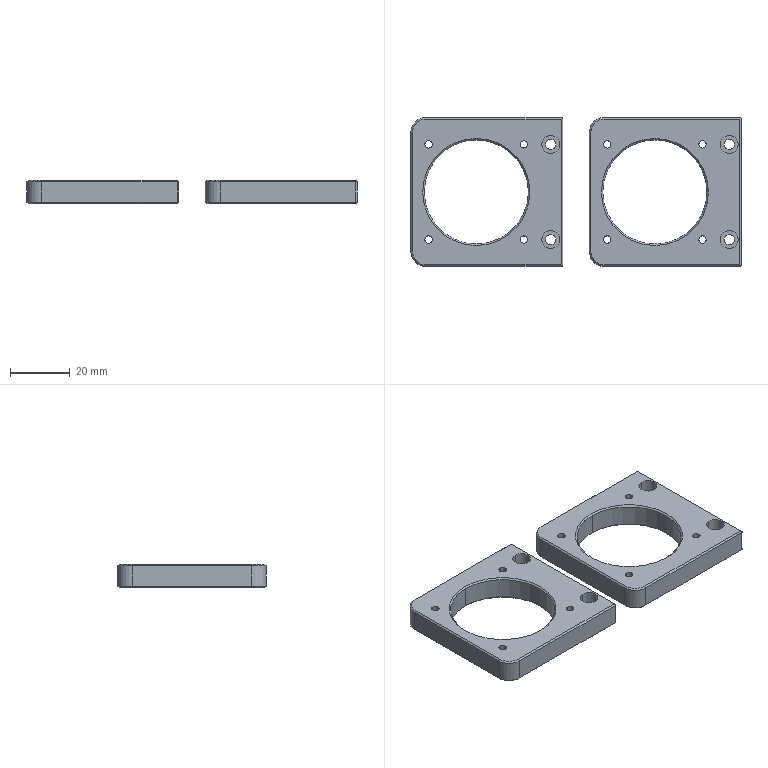Part | 2 solids | 104 faces | box 111 x 50 x 8 mm | volume 24121 mm3 | cylinder 44 | plane 32 | cone 28 | commonest cylinder face diameters 2.5 x16 3.5 x8 6 x8 1 x4 10 x4 35 x4